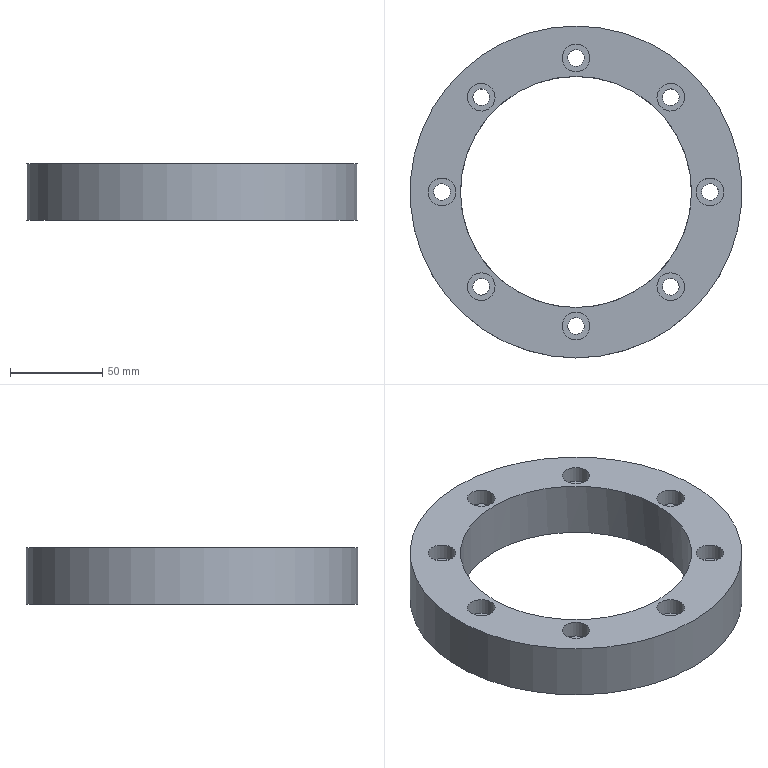Part | NX | features 5003_106_Bearing with gear 2 | 1 solid | 28 faces | box 179.5 x 179.5 x 30.5 mm | volume 373868 mm3 | cylinder 18 | plane 10 | commonest cylinder face diameters 9 x8 15 x8 125 x1 179.5 x1
STEP:
#1=CARTESIAN_POINT('',(66.525,-322.,-216.5));
#2=VERTEX_POINT('',#1);
#3=CARTESIAN_POINT('',(71.025,-322.,-216.5));
#4=DIRECTION('',(0.,0.,1.));
#5=DIRECTION('',(-1.,0.,0.));
#6=AXIS2_PLACEMENT_3D('',#3,#4,#5);
#7=CIRCLE('',#6,4.5);
#8=EDGE_CURVE('',#2,#2,#7,.T.);
#9=ORIENTED_EDGE('',*,*,#8,.T.);
#10=EDGE_LOOP('',(#9));
#11=FACE_BOUND('',#10,.T.);
#12=CARTESIAN_POINT('',(71.025,-317.5,-238.));
#13=VERTEX_POINT('',#12);
#14=CARTESIAN_POINT('',(71.025,-322.,-238.));
#15=DIRECTION('',(0.,0.,-1.));
#16=DIRECTION('',(0.,1.,0.));
#17=AXIS2_PLACEMENT_3D('',#14,#15,#16);
#18=CIRCLE('',#17,4.5);
#19=EDGE_CURVE('',#13,#13,#18,.T.);
#20=ORIENTED_EDGE('',*,*,#19,.T.);
#21=EDGE_LOOP('',(#20));
#22=FACE_BOUND('',#21,.T.);
#23=CARTESIAN_POINT('',(71.025,-322.,-207.5));
#24=DIRECTION('',(0.,0.,1.));
#25=DIRECTION('',(-1.,0.,0.));
#26=AXIS2_PLACEMENT_3D('',#23,#24,#25);
#27=CYLINDRICAL_SURFACE('',#26,4.5);
#28=ADVANCED_FACE('',(#11,#22),#27,.F.);
#29=CARTESIAN_POINT('',(46.608,-370.083,-216.5));
#30=VERTEX_POINT('',#29);
#31=CARTESIAN_POINT('',(49.79,-373.265,-216.5));
#32=DIRECTION('',(0.,0.,1.));
#33=DIRECTION('',(-0.7071,0.7071,0.));
#34=AXIS2_PLACEMENT_3D('',#31,#32,#33);
#35=CIRCLE('',#34,4.5);
#36=EDGE_CURVE('',#30,#30,#35,.T.);
#37=ORIENTED_EDGE('',*,*,#36,.T.);
#38=EDGE_LOOP('',(#37));
#39=FACE_BOUND('',#38,.T.);
#40=CARTESIAN_POINT('',(52.972,-370.083,-238.));
#41=VERTEX_POINT('',#40);
#42=CARTESIAN_POINT('',(49.79,-373.265,-238.));
#43=DIRECTION('',(0.,0.,-1.));
#44=DIRECTION('',(0.7071,0.7071,0.));
#45=AXIS2_PLACEMENT_3D('',#42,#43,#44);
#46=CIRCLE('',#45,4.5);
#47=EDGE_CURVE('',#41,#41,#46,.T.);
#48=ORIENTED_EDGE('',*,*,#47,.T.);
#49=EDGE_LOOP('',(#48));
#50=FACE_BOUND('',#49,.T.);
#51=CARTESIAN_POINT('',(49.79,-373.265,-207.5));
#52=DIRECTION('',(0.,0.,1.));
#53=DIRECTION('',(-0.7071,0.7071,0.));
#54=AXIS2_PLACEMENT_3D('',#51,#52,#53);
#55=CYLINDRICAL_SURFACE('',#54,4.5);
#56=ADVANCED_FACE('',(#39,#50),#55,.F.);
#57=CARTESIAN_POINT('',(-1.475,-390.,-216.5));
#58=VERTEX_POINT('',#57);
#59=CARTESIAN_POINT('',(-1.475,-394.5,-216.5));
#60=DIRECTION('',(0.,0.,1.));
#61=DIRECTION('',(0.,1.,0.));
#62=AXIS2_PLACEMENT_3D('',#59,#60,#61);
#63=CIRCLE('',#62,4.5);
#64=EDGE_CURVE('',#58,#58,#63,.T.);
#65=ORIENTED_EDGE('',*,*,#64,.T.);
#66=EDGE_LOOP('',(#65));
#67=FACE_BOUND('',#66,.T.);
#68=CARTESIAN_POINT('',(3.025,-394.5,-238.));
#69=VERTEX_POINT('',#68);
#70=CARTESIAN_POINT('',(-1.475,-394.5,-238.));
#71=DIRECTION('',(0.,0.,-1.));
#72=DIRECTION('',(1.,0.,0.));
#73=AXIS2_PLACEMENT_3D('',#70,#71,#72);
#74=CIRCLE('',#73,4.5);
#75=EDGE_CURVE('',#69,#69,#74,.T.);
#76=ORIENTED_EDGE('',*,*,#75,.T.);
#77=EDGE_LOOP('',(#76));
#78=FACE_BOUND('',#77,.T.);
#79=CARTESIAN_POINT('',(-1.475,-394.5,-207.5));
#80=DIRECTION('',(0.,0.,1.));
#81=DIRECTION('',(0.,1.,0.));
#82=AXIS2_PLACEMENT_3D('',#79,#80,#81);
#83=CYLINDRICAL_SURFACE('',#82,4.5);
#84=ADVANCED_FACE('',(#67,#78),#83,.F.);
#85=CARTESIAN_POINT('',(-49.558,-370.083,-216.5));
#86=VERTEX_POINT('',#85);
#87=CARTESIAN_POINT('',(-52.74,-373.265,-216.5));
#88=DIRECTION('',(0.,0.,1.));
#89=DIRECTION('',(0.7071,0.7071,0.));
#90=AXIS2_PLACEMENT_3D('',#87,#88,#89);
#91=CIRCLE('',#90,4.5);
#92=EDGE_CURVE('',#86,#86,#91,.T.);
#93=ORIENTED_EDGE('',*,*,#92,.T.);
#94=EDGE_LOOP('',(#93));
#95=FACE_BOUND('',#94,.T.);
#96=CARTESIAN_POINT('',(-49.558,-376.447,-238.));
#97=VERTEX_POINT('',#96);
#98=CARTESIAN_POINT('',(-52.74,-373.265,-238.));
#99=DIRECTION('',(0.,0.,-1.));
#100=DIRECTION('',(0.7071,-0.7071,0.));
#101=AXIS2_PLACEMENT_3D('',#98,#99,#100);
#102=CIRCLE('',#101,4.5);
#103=EDGE_CURVE('',#97,#97,#102,.T.);
#104=ORIENTED_EDGE('',*,*,#103,.T.);
#105=EDGE_LOOP('',(#104));
#106=FACE_BOUND('',#105,.T.);
#107=CARTESIAN_POINT('',(-52.74,-373.265,-207.5));
#108=DIRECTION('',(0.,0.,1.));
#109=DIRECTION('',(0.7071,0.7071,0.));
#110=AXIS2_PLACEMENT_3D('',#107,#108,#109);
#111=CYLINDRICAL_SURFACE('',#110,4.5);
#112=ADVANCED_FACE('',(#95,#106),#111,.F.);
#113=CARTESIAN_POINT('',(-69.475,-322.,-216.5));
#114=VERTEX_POINT('',#113);
#115=CARTESIAN_POINT('',(-73.975,-322.,-216.5));
#116=DIRECTION('',(0.,0.,1.));
#117=DIRECTION('',(1.,0.,0.));
#118=AXIS2_PLACEMENT_3D('',#115,#116,#117);
#119=CIRCLE('',#118,4.5);
#120=EDGE_CURVE('',#114,#114,#119,.T.);
#121=ORIENTED_EDGE('',*,*,#120,.T.);
#122=EDGE_LOOP('',(#121));
#123=FACE_BOUND('',#122,.T.);
#124=CARTESIAN_POINT('',(-73.975,-326.5,-238.));
#125=VERTEX_POINT('',#124);
#126=CARTESIAN_POINT('',(-73.975,-322.,-238.));
#127=DIRECTION('',(0.,0.,-1.));
#128=DIRECTION('',(0.,-1.,0.));
#129=AXIS2_PLACEMENT_3D('',#126,#127,#128);
#130=CIRCLE('',#129,4.5);
#131=EDGE_CURVE('',#125,#125,#130,.T.);
#132=ORIENTED_EDGE('',*,*,#131,.T.);
#133=EDGE_LOOP('',(#132));
#134=FACE_BOUND('',#133,.T.);
#135=CARTESIAN_POINT('',(-73.975,-322.,-207.5));
#136=DIRECTION('',(0.,0.,1.));
#137=DIRECTION('',(1.,0.,0.));
#138=AXIS2_PLACEMENT_3D('',#135,#136,#137);
#139=CYLINDRICAL_SURFACE('',#138,4.5);
#140=ADVANCED_FACE('',(#123,#134),#139,.F.);
#141=CARTESIAN_POINT('',(-49.558,-273.917,-216.5));
#142=VERTEX_POINT('',#141);
#143=CARTESIAN_POINT('',(-52.74,-270.735,-216.5));
#144=DIRECTION('',(0.,0.,1.));
#145=DIRECTION('',(0.7071,-0.7071,0.));
#146=AXIS2_PLACEMENT_3D('',#143,#144,#145);
#147=CIRCLE('',#146,4.5);
#148=EDGE_CURVE('',#142,#142,#147,.T.);
#149=ORIENTED_EDGE('',*,*,#148,.T.);
#150=EDGE_LOOP('',(#149));
#151=FACE_BOUND('',#150,.T.);
#152=CARTESIAN_POINT('',(-55.922,-273.917,-238.));
#153=VERTEX_POINT('',#152);
#154=CARTESIAN_POINT('',(-52.74,-270.735,-238.));
#155=DIRECTION('',(0.,0.,-1.));
#156=DIRECTION('',(-0.7071,-0.7071,0.));
#157=AXIS2_PLACEMENT_3D('',#154,#155,#156);
#158=CIRCLE('',#157,4.5);
#159=EDGE_CURVE('',#153,#153,#158,.T.);
#160=ORIENTED_EDGE('',*,*,#159,.T.);
#161=EDGE_LOOP('',(#160));
#162=FACE_BOUND('',#161,.T.);
#163=CARTESIAN_POINT('',(-52.74,-270.735,-207.5));
#164=DIRECTION('',(0.,0.,1.));
#165=DIRECTION('',(0.7071,-0.7071,0.));
#166=AXIS2_PLACEMENT_3D('',#163,#164,#165);
#167=CYLINDRICAL_SURFACE('',#166,4.5);
#168=ADVANCED_FACE('',(#151,#162),#167,.F.);
#169=CARTESIAN_POINT('',(-1.475,-254.,-216.5));
#170=VERTEX_POINT('',#169);
#171=CARTESIAN_POINT('',(-1.475,-249.5,-216.5));
#172=DIRECTION('',(0.,0.,1.));
#173=DIRECTION('',(0.,-1.,0.));
#174=AXIS2_PLACEMENT_3D('',#171,#172,#173);
#175=CIRCLE('',#174,4.5);
#176=EDGE_CURVE('',#170,#170,#175,.T.);
#177=ORIENTED_EDGE('',*,*,#176,.T.);
#178=EDGE_LOOP('',(#177));
#179=FACE_BOUND('',#178,.T.);
#180=CARTESIAN_POINT('',(-5.975,-249.5,-238.));
#181=VERTEX_POINT('',#180);
#182=CARTESIAN_POINT('',(-1.475,-249.5,-238.));
#183=DIRECTION('',(0.,0.,-1.));
#184=DIRECTION('',(-1.,0.,0.));
#185=AXIS2_PLACEMENT_3D('',#182,#183,#184);
#186=CIRCLE('',#185,4.5);
#187=EDGE_CURVE('',#181,#181,#186,.T.);
#188=ORIENTED_EDGE('',*,*,#187,.T.);
#189=EDGE_LOOP('',(#188));
#190=FACE_BOUND('',#189,.T.);
#191=CARTESIAN_POINT('',(-1.475,-249.5,-207.5));
#192=DIRECTION('',(0.,0.,1.));
#193=DIRECTION('',(0.,-1.,0.));
#194=AXIS2_PLACEMENT_3D('',#191,#192,#193);
#195=CYLINDRICAL_SURFACE('',#194,4.5);
#196=ADVANCED_FACE('',(#179,#190),#195,.F.);
#197=CARTESIAN_POINT('',(46.608,-273.917,-216.5));
#198=VERTEX_POINT('',#197);
#199=CARTESIAN_POINT('',(49.79,-270.735,-216.5));
#200=DIRECTION('',(0.,0.,1.));
#201=DIRECTION('',(-0.7071,-0.7071,0.));
#202=AXIS2_PLACEMENT_3D('',#199,#200,#201);
#203=CIRCLE('',#202,4.5);
#204=EDGE_CURVE('',#198,#198,#203,.T.);
#205=ORIENTED_EDGE('',*,*,#204,.T.);
#206=EDGE_LOOP('',(#205));
#207=FACE_BOUND('',#206,.T.);
#208=CARTESIAN_POINT('',(46.608,-267.553,-238.));
#209=VERTEX_POINT('',#208);
#210=CARTESIAN_POINT('',(49.79,-270.735,-238.));
#211=DIRECTION('',(0.,0.,-1.));
#212=DIRECTION('',(-0.7071,0.7071,0.));
#213=AXIS2_PLACEMENT_3D('',#210,#211,#212);
#214=CIRCLE('',#213,4.5);
#215=EDGE_CURVE('',#209,#209,#214,.T.);
#216=ORIENTED_EDGE('',*,*,#215,.T.);
#217=EDGE_LOOP('',(#216));
#218=FACE_BOUND('',#217,.T.);
#219=CARTESIAN_POINT('',(49.79,-270.735,-207.5));
#220=DIRECTION('',(0.,0.,1.));
#221=DIRECTION('',(-0.7071,-0.7071,0.));
#222=AXIS2_PLACEMENT_3D('',#219,#220,#221);
#223=CYLINDRICAL_SURFACE('',#222,4.5);
#224=ADVANCED_FACE('',(#207,#218),#223,.F.);
#225=ORIENTED_EDGE('',*,*,#8,.F.);
#226=EDGE_LOOP('',(#225));
#227=FACE_BOUND('',#226,.T.);
#228=CARTESIAN_POINT('',(63.525,-322.,-216.5));
#229=VERTEX_POINT('',#228);
#230=CARTESIAN_POINT('',(71.025,-322.,-216.5));
#231=DIRECTION('',(0.,0.,1.));
#232=DIRECTION('',(-1.,0.,0.));
#233=AXIS2_PLACEMENT_3D('',#230,#231,#232);
#234=CIRCLE('',#233,7.5);
#235=EDGE_CURVE('',#229,#229,#234,.T.);
#236=ORIENTED_EDGE('',*,*,#235,.T.);
#237=EDGE_LOOP('',(#236));
#238=FACE_BOUND('',#237,.T.);
#239=CARTESIAN_POINT('',(71.025,-326.5,-216.5));
#240=DIRECTION('',(0.,0.,-1.));
#241=DIRECTION('',(1.,0.,0.));
#242=AXIS2_PLACEMENT_3D('',#239,#240,#241);
#243=PLANE('',#242);
#244=ADVANCED_FACE('',(#227,#238),#243,.F.);
#245=ORIENTED_EDGE('',*,*,#36,.F.);
#246=EDGE_LOOP('',(#245));
#247=FACE_BOUND('',#246,.T.);
#248=CARTESIAN_POINT('',(44.487,-367.962,-216.5));
#249=VERTEX_POINT('',#248);
#250=CARTESIAN_POINT('',(49.79,-373.265,-216.5));
#251=DIRECTION('',(0.,0.,1.));
#252=DIRECTION('',(-0.7071,0.7071,0.));
#253=AXIS2_PLACEMENT_3D('',#250,#251,#252);
#254=CIRCLE('',#253,7.5);
#255=EDGE_CURVE('',#249,#249,#254,.T.);
#256=ORIENTED_EDGE('',*,*,#255,.T.);
#257=EDGE_LOOP('',(#256));
#258=FACE_BOUND('',#257,.T.);
#259=CARTESIAN_POINT('',(46.608,-376.447,-216.5));
#260=DIRECTION('',(0.,0.,-1.));
#261=DIRECTION('',(0.7071,-0.7071,0.));
#262=AXIS2_PLACEMENT_3D('',#259,#260,#261);
#263=PLANE('',#262);
#264=ADVANCED_FACE('',(#247,#258),#263,.F.);
#265=ORIENTED_EDGE('',*,*,#64,.F.);
#266=EDGE_LOOP('',(#265));
#267=FACE_BOUND('',#266,.T.);
#268=CARTESIAN_POINT('',(-1.475,-387.,-216.5));
#269=VERTEX_POINT('',#268);
#270=CARTESIAN_POINT('',(-1.475,-394.5,-216.5));
#271=DIRECTION('',(0.,0.,1.));
#272=DIRECTION('',(0.,1.,0.));
#273=AXIS2_PLACEMENT_3D('',#270,#271,#272);
#274=CIRCLE('',#273,7.5);
#275=EDGE_CURVE('',#269,#269,#274,.T.);
#276=ORIENTED_EDGE('',*,*,#275,.T.);
#277=EDGE_LOOP('',(#276));
#278=FACE_BOUND('',#277,.T.);
#279=CARTESIAN_POINT('',(-5.975,-394.5,-216.5));
#280=DIRECTION('',(0.,0.,-1.));
#281=DIRECTION('',(0.,-1.,0.));
#282=AXIS2_PLACEMENT_3D('',#279,#280,#281);
#283=PLANE('',#282);
#284=ADVANCED_FACE('',(#267,#278),#283,.F.);
#285=ORIENTED_EDGE('',*,*,#92,.F.);
#286=EDGE_LOOP('',(#285));
#287=FACE_BOUND('',#286,.T.);
#288=CARTESIAN_POINT('',(-47.437,-367.962,-216.5));
#289=VERTEX_POINT('',#288);
#290=CARTESIAN_POINT('',(-52.74,-373.265,-216.5));
#291=DIRECTION('',(0.,0.,1.));
#292=DIRECTION('',(0.7071,0.7071,0.));
#293=AXIS2_PLACEMENT_3D('',#290,#291,#292);
#294=CIRCLE('',#293,7.5);
#295=EDGE_CURVE('',#289,#289,#294,.T.);
#296=ORIENTED_EDGE('',*,*,#295,.T.);
#297=EDGE_LOOP('',(#296));
#298=FACE_BOUND('',#297,.T.);
#299=CARTESIAN_POINT('',(-55.922,-370.083,-216.5));
#300=DIRECTION('',(0.,0.,-1.));
#301=DIRECTION('',(-0.7071,-0.7071,0.));
#302=AXIS2_PLACEMENT_3D('',#299,#300,#301);
#303=PLANE('',#302);
#304=ADVANCED_FACE('',(#287,#298),#303,.F.);
#305=ORIENTED_EDGE('',*,*,#120,.F.);
#306=EDGE_LOOP('',(#305));
#307=FACE_BOUND('',#306,.T.);
#308=CARTESIAN_POINT('',(-66.475,-322.,-216.5));
#309=VERTEX_POINT('',#308);
#310=CARTESIAN_POINT('',(-73.975,-322.,-216.5));
#311=DIRECTION('',(0.,0.,1.));
#312=DIRECTION('',(1.,0.,0.));
#313=AXIS2_PLACEMENT_3D('',#310,#311,#312);
#314=CIRCLE('',#313,7.5);
#315=EDGE_CURVE('',#309,#309,#314,.T.);
#316=ORIENTED_EDGE('',*,*,#315,.T.);
#317=EDGE_LOOP('',(#316));
#318=FACE_BOUND('',#317,.T.);
#319=CARTESIAN_POINT('',(-73.975,-317.5,-216.5));
#320=DIRECTION('',(0.,0.,-1.));
#321=DIRECTION('',(-1.,0.,0.));
#322=AXIS2_PLACEMENT_3D('',#319,#320,#321);
#323=PLANE('',#322);
#324=ADVANCED_FACE('',(#307,#318),#323,.F.);
#325=ORIENTED_EDGE('',*,*,#148,.F.);
#326=EDGE_LOOP('',(#325));
#327=FACE_BOUND('',#326,.T.);
#328=CARTESIAN_POINT('',(-47.437,-276.038,-216.5));
#329=VERTEX_POINT('',#328);
#330=CARTESIAN_POINT('',(-52.74,-270.735,-216.5));
#331=DIRECTION('',(0.,0.,1.));
#332=DIRECTION('',(0.7071,-0.7071,0.));
#333=AXIS2_PLACEMENT_3D('',#330,#331,#332);
#334=CIRCLE('',#333,7.5);
#335=EDGE_CURVE('',#329,#329,#334,.T.);
#336=ORIENTED_EDGE('',*,*,#335,.T.);
#337=EDGE_LOOP('',(#336));
#338=FACE_BOUND('',#337,.T.);
#339=CARTESIAN_POINT('',(-49.558,-267.553,-216.5));
#340=DIRECTION('',(0.,0.,-1.));
#341=DIRECTION('',(-0.7071,0.7071,0.));
#342=AXIS2_PLACEMENT_3D('',#339,#340,#341);
#343=PLANE('',#342);
#344=ADVANCED_FACE('',(#327,#338),#343,.F.);
#345=ORIENTED_EDGE('',*,*,#176,.F.);
#346=EDGE_LOOP('',(#345));
#347=FACE_BOUND('',#346,.T.);
#348=CARTESIAN_POINT('',(-1.475,-257.,-216.5));
#349=VERTEX_POINT('',#348);
#350=CARTESIAN_POINT('',(-1.475,-249.5,-216.5));
#351=DIRECTION('',(0.,0.,1.));
#352=DIRECTION('',(0.,-1.,0.));
#353=AXIS2_PLACEMENT_3D('',#350,#351,#352);
#354=CIRCLE('',#353,7.5);
#355=EDGE_CURVE('',#349,#349,#354,.T.);
#356=ORIENTED_EDGE('',*,*,#355,.T.);
#357=EDGE_LOOP('',(#356));
#358=FACE_BOUND('',#357,.T.);
#359=CARTESIAN_POINT('',(3.025,-249.5,-216.5));
#360=DIRECTION('',(0.,0.,-1.));
#361=DIRECTION('',(0.,1.,0.));
#362=AXIS2_PLACEMENT_3D('',#359,#360,#361);
#363=PLANE('',#362);
#364=ADVANCED_FACE('',(#347,#358),#363,.F.);
#365=ORIENTED_EDGE('',*,*,#204,.F.);
#366=EDGE_LOOP('',(#365));
#367=FACE_BOUND('',#366,.T.);
#368=CARTESIAN_POINT('',(44.487,-276.038,-216.5));
#369=VERTEX_POINT('',#368);
#370=CARTESIAN_POINT('',(49.79,-270.735,-216.5));
#371=DIRECTION('',(0.,0.,1.));
#372=DIRECTION('',(-0.7071,-0.7071,0.));
#373=AXIS2_PLACEMENT_3D('',#370,#371,#372);
#374=CIRCLE('',#373,7.5);
#375=EDGE_CURVE('',#369,#369,#374,.T.);
#376=ORIENTED_EDGE('',*,*,#375,.T.);
#377=EDGE_LOOP('',(#376));
#378=FACE_BOUND('',#377,.T.);
#379=CARTESIAN_POINT('',(52.972,-273.917,-216.5));
#380=DIRECTION('',(0.,0.,-1.));
#381=DIRECTION('',(0.7071,0.7071,0.));
#382=AXIS2_PLACEMENT_3D('',#379,#380,#381);
#383=PLANE('',#382);
#384=ADVANCED_FACE('',(#367,#378),#383,.F.);
#385=CARTESIAN_POINT('',(-1.475,-259.5,-238.));
#386=VERTEX_POINT('',#385);
#387=CARTESIAN_POINT('',(-1.475,-322.,-238.));
#388=DIRECTION('',(0.,0.,-1.));
#389=DIRECTION('',(0.,1.,0.));
#390=AXIS2_PLACEMENT_3D('',#387,#388,#389);
#391=CIRCLE('',#390,62.5);
#392=EDGE_CURVE('',#386,#386,#391,.T.);
#393=ORIENTED_EDGE('',*,*,#392,.T.);
#394=EDGE_LOOP('',(#393));
#395=FACE_BOUND('',#394,.T.);
#396=CARTESIAN_POINT('',(-1.475,-384.5,-207.5));
#397=VERTEX_POINT('',#396);
#398=CARTESIAN_POINT('',(-1.475,-322.,-207.5));
#399=DIRECTION('',(0.,0.,1.));
#400=DIRECTION('',(0.,-1.,0.));
#401=AXIS2_PLACEMENT_3D('',#398,#399,#400);
#402=CIRCLE('',#401,62.5);
#403=EDGE_CURVE('',#397,#397,#402,.F.);
#404=ORIENTED_EDGE('',*,*,#403,.F.);
#405=EDGE_LOOP('',(#404));
#406=FACE_BOUND('',#405,.T.);
#407=CARTESIAN_POINT('',(-1.475,-322.,-202.));
#408=DIRECTION('',(0.,0.,-1.));
#409=DIRECTION('',(0.,1.,0.));
#410=AXIS2_PLACEMENT_3D('',#407,#408,#409);
#411=CYLINDRICAL_SURFACE('',#410,62.5);
#412=ADVANCED_FACE('',(#395,#406),#411,.F.);
#413=ORIENTED_EDGE('',*,*,#235,.F.);
#414=EDGE_LOOP('',(#413));
#415=FACE_BOUND('',#414,.T.);
#416=CARTESIAN_POINT('',(63.525,-322.,-207.5));
#417=VERTEX_POINT('',#416);
#418=CARTESIAN_POINT('',(71.025,-322.,-207.5));
#419=DIRECTION('',(0.,0.,1.));
#420=DIRECTION('',(-1.,0.,0.));
#421=AXIS2_PLACEMENT_3D('',#418,#419,#420);
#422=CIRCLE('',#421,7.5);
#423=EDGE_CURVE('',#417,#417,#422,.T.);
#424=ORIENTED_EDGE('',*,*,#423,.T.);
#425=EDGE_LOOP('',(#424));
#426=FACE_BOUND('',#425,.T.);
#427=CARTESIAN_POINT('',(71.025,-322.,-207.5));
#428=DIRECTION('',(0.,0.,1.));
#429=DIRECTION('',(-1.,0.,0.));
#430=AXIS2_PLACEMENT_3D('',#427,#428,#429);
#431=CYLINDRICAL_SURFACE('',#430,7.5);
#432=ADVANCED_FACE('',(#415,#426),#431,.F.);
#433=ORIENTED_EDGE('',*,*,#255,.F.);
#434=EDGE_LOOP('',(#433));
#435=FACE_BOUND('',#434,.T.);
#436=CARTESIAN_POINT('',(44.487,-367.962,-207.5));
#437=VERTEX_POINT('',#436);
#438=CARTESIAN_POINT('',(49.79,-373.265,-207.5));
#439=DIRECTION('',(0.,0.,1.));
#440=DIRECTION('',(-0.7071,0.7071,0.));
#441=AXIS2_PLACEMENT_3D('',#438,#439,#440);
#442=CIRCLE('',#441,7.5);
#443=EDGE_CURVE('',#437,#437,#442,.T.);
#444=ORIENTED_EDGE('',*,*,#443,.T.);
#445=EDGE_LOOP('',(#444));
#446=FACE_BOUND('',#445,.T.);
#447=CARTESIAN_POINT('',(49.79,-373.265,-207.5));
#448=DIRECTION('',(0.,0.,1.));
#449=DIRECTION('',(-0.7071,0.7071,0.));
#450=AXIS2_PLACEMENT_3D('',#447,#448,#449);
#451=CYLINDRICAL_SURFACE('',#450,7.5);
#452=ADVANCED_FACE('',(#435,#446),#451,.F.);
#453=ORIENTED_EDGE('',*,*,#275,.F.);
#454=EDGE_LOOP('',(#453));
#455=FACE_BOUND('',#454,.T.);
#456=CARTESIAN_POINT('',(-1.475,-387.,-207.5));
#457=VERTEX_POINT('',#456);
#458=CARTESIAN_POINT('',(-1.475,-394.5,-207.5));
#459=DIRECTION('',(0.,0.,1.));
#460=DIRECTION('',(0.,1.,0.));
#461=AXIS2_PLACEMENT_3D('',#458,#459,#460);
#462=CIRCLE('',#461,7.5);
#463=EDGE_CURVE('',#457,#457,#462,.T.);
#464=ORIENTED_EDGE('',*,*,#463,.T.);
#465=EDGE_LOOP('',(#464));
#466=FACE_BOUND('',#465,.T.);
#467=CARTESIAN_POINT('',(-1.475,-394.5,-207.5));
#468=DIRECTION('',(0.,0.,1.));
#469=DIRECTION('',(0.,1.,0.));
#470=AXIS2_PLACEMENT_3D('',#467,#468,#469);
#471=CYLINDRICAL_SURFACE('',#470,7.5);
#472=ADVANCED_FACE('',(#455,#466),#471,.F.);
#473=ORIENTED_EDGE('',*,*,#295,.F.);
#474=EDGE_LOOP('',(#473));
#475=FACE_BOUND('',#474,.T.);
#476=CARTESIAN_POINT('',(-47.437,-367.962,-207.5));
#477=VERTEX_POINT('',#476);
#478=CARTESIAN_POINT('',(-52.74,-373.265,-207.5));
#479=DIRECTION('',(0.,0.,1.));
#480=DIRECTION('',(0.7071,0.7071,0.));
#481=AXIS2_PLACEMENT_3D('',#478,#479,#480);
#482=CIRCLE('',#481,7.5);
#483=EDGE_CURVE('',#477,#477,#482,.T.);
#484=ORIENTED_EDGE('',*,*,#483,.T.);
#485=EDGE_LOOP('',(#484));
#486=FACE_BOUND('',#485,.T.);
#487=CARTESIAN_POINT('',(-52.74,-373.265,-207.5));
#488=DIRECTION('',(0.,0.,1.));
#489=DIRECTION('',(0.7071,0.7071,0.));
#490=AXIS2_PLACEMENT_3D('',#487,#488,#489);
#491=CYLINDRICAL_SURFACE('',#490,7.5);
#492=ADVANCED_FACE('',(#475,#486),#491,.F.);
#493=ORIENTED_EDGE('',*,*,#315,.F.);
#494=EDGE_LOOP('',(#493));
#495=FACE_BOUND('',#494,.T.);
#496=CARTESIAN_POINT('',(-66.475,-322.,-207.5));
#497=VERTEX_POINT('',#496);
#498=CARTESIAN_POINT('',(-73.975,-322.,-207.5));
#499=DIRECTION('',(0.,0.,1.));
#500=DIRECTION('',(1.,0.,0.));
#501=AXIS2_PLACEMENT_3D('',#498,#499,#500);
#502=CIRCLE('',#501,7.5);
#503=EDGE_CURVE('',#497,#497,#502,.T.);
#504=ORIENTED_EDGE('',*,*,#503,.T.);
#505=EDGE_LOOP('',(#504));
#506=FACE_BOUND('',#505,.T.);
#507=CARTESIAN_POINT('',(-73.975,-322.,-207.5));
#508=DIRECTION('',(0.,0.,1.));
#509=DIRECTION('',(1.,0.,0.));
#510=AXIS2_PLACEMENT_3D('',#507,#508,#509);
#511=CYLINDRICAL_SURFACE('',#510,7.5);
#512=ADVANCED_FACE('',(#495,#506),#511,.F.);
#513=ORIENTED_EDGE('',*,*,#335,.F.);
#514=EDGE_LOOP('',(#513));
#515=FACE_BOUND('',#514,.T.);
#516=CARTESIAN_POINT('',(-47.437,-276.038,-207.5));
#517=VERTEX_POINT('',#516);
#518=CARTESIAN_POINT('',(-52.74,-270.735,-207.5));
#519=DIRECTION('',(0.,0.,1.));
#520=DIRECTION('',(0.7071,-0.7071,0.));
#521=AXIS2_PLACEMENT_3D('',#518,#519,#520);
#522=CIRCLE('',#521,7.5);
#523=EDGE_CURVE('',#517,#517,#522,.T.);
#524=ORIENTED_EDGE('',*,*,#523,.T.);
#525=EDGE_LOOP('',(#524));
#526=FACE_BOUND('',#525,.T.);
#527=CARTESIAN_POINT('',(-52.74,-270.735,-207.5));
#528=DIRECTION('',(0.,0.,1.));
#529=DIRECTION('',(0.7071,-0.7071,0.));
#530=AXIS2_PLACEMENT_3D('',#527,#528,#529);
#531=CYLINDRICAL_SURFACE('',#530,7.5);
#532=ADVANCED_FACE('',(#515,#526),#531,.F.);
#533=ORIENTED_EDGE('',*,*,#355,.F.);
#534=EDGE_LOOP('',(#533));
#535=FACE_BOUND('',#534,.T.);
#536=CARTESIAN_POINT('',(-1.475,-257.,-207.5));
#537=VERTEX_POINT('',#536);
#538=CARTESIAN_POINT('',(-1.475,-249.5,-207.5));
#539=DIRECTION('',(0.,0.,1.));
#540=DIRECTION('',(0.,-1.,0.));
#541=AXIS2_PLACEMENT_3D('',#538,#539,#540);
#542=CIRCLE('',#541,7.5);
#543=EDGE_CURVE('',#537,#537,#542,.T.);
#544=ORIENTED_EDGE('',*,*,#543,.T.);
#545=EDGE_LOOP('',(#544));
#546=FACE_BOUND('',#545,.T.);
#547=CARTESIAN_POINT('',(-1.475,-249.5,-207.5));
#548=DIRECTION('',(0.,0.,1.));
#549=DIRECTION('',(0.,-1.,0.));
#550=AXIS2_PLACEMENT_3D('',#547,#548,#549);
#551=CYLINDRICAL_SURFACE('',#550,7.5);
#552=ADVANCED_FACE('',(#535,#546),#551,.F.);
#553=ORIENTED_EDGE('',*,*,#375,.F.);
#554=EDGE_LOOP('',(#553));
#555=FACE_BOUND('',#554,.T.);
#556=CARTESIAN_POINT('',(44.487,-276.038,-207.5));
#557=VERTEX_POINT('',#556);
#558=CARTESIAN_POINT('',(49.79,-270.735,-207.5));
#559=DIRECTION('',(0.,0.,1.));
#560=DIRECTION('',(-0.7071,-0.7071,0.));
#561=AXIS2_PLACEMENT_3D('',#558,#559,#560);
#562=CIRCLE('',#561,7.5);
#563=EDGE_CURVE('',#557,#557,#562,.T.);
#564=ORIENTED_EDGE('',*,*,#563,.T.);
#565=EDGE_LOOP('',(#564));
#566=FACE_BOUND('',#565,.T.);
#567=CARTESIAN_POINT('',(49.79,-270.735,-207.5));
#568=DIRECTION('',(0.,0.,1.));
#569=DIRECTION('',(-0.7071,-0.7071,0.));
#570=AXIS2_PLACEMENT_3D('',#567,#568,#569);
#571=CYLINDRICAL_SURFACE('',#570,7.5);
#572=ADVANCED_FACE('',(#555,#566),#571,.F.);
#573=ORIENTED_EDGE('',*,*,#563,.F.);
#574=EDGE_LOOP('',(#573));
#575=FACE_BOUND('',#574,.T.);
#576=ORIENTED_EDGE('',*,*,#543,.F.);
#577=EDGE_LOOP('',(#576));
#578=FACE_BOUND('',#577,.T.);
#579=ORIENTED_EDGE('',*,*,#523,.F.);
#580=EDGE_LOOP('',(#579));
#581=FACE_BOUND('',#580,.T.);
#582=ORIENTED_EDGE('',*,*,#503,.F.);
#583=EDGE_LOOP('',(#582));
#584=FACE_BOUND('',#583,.T.);
#585=ORIENTED_EDGE('',*,*,#483,.F.);
#586=EDGE_LOOP('',(#585));
#587=FACE_BOUND('',#586,.T.);
#588=ORIENTED_EDGE('',*,*,#463,.F.);
#589=EDGE_LOOP('',(#588));
#590=FACE_BOUND('',#589,.T.);
#591=ORIENTED_EDGE('',*,*,#443,.F.);
#592=EDGE_LOOP('',(#591));
#593=FACE_BOUND('',#592,.T.);
#594=ORIENTED_EDGE('',*,*,#423,.F.);
#595=EDGE_LOOP('',(#594));
#596=FACE_BOUND('',#595,.T.);
#597=CARTESIAN_POINT('',(-1.475,-411.75,-207.5));
#598=VERTEX_POINT('',#597);
#599=CARTESIAN_POINT('',(-1.475,-322.,-207.5));
#600=DIRECTION('',(0.,0.,1.));
#601=DIRECTION('',(0.,-1.,0.));
#602=AXIS2_PLACEMENT_3D('',#599,#600,#601);
#603=CIRCLE('',#602,89.75);
#604=EDGE_CURVE('',#598,#598,#603,.T.);
#605=ORIENTED_EDGE('',*,*,#604,.T.);
#606=EDGE_LOOP('',(#605));
#607=FACE_BOUND('',#606,.T.);
#608=ORIENTED_EDGE('',*,*,#403,.T.);
#609=EDGE_LOOP('',(#608));
#610=FACE_BOUND('',#609,.T.);
#611=CARTESIAN_POINT('',(-1.475,-322.,-207.5));
#612=DIRECTION('',(0.,0.,1.));
#613=DIRECTION('',(0.,-1.,0.));
#614=AXIS2_PLACEMENT_3D('',#611,#612,#613);
#615=PLANE('',#614);
#616=ADVANCED_FACE('',(#575,#578,#581,#584,#587,#590,#593,#596,#607,#610),#615,.T.);
#617=ORIENTED_EDGE('',*,*,#215,.F.);
#618=EDGE_LOOP('',(#617));
#619=FACE_BOUND('',#618,.T.);
#620=ORIENTED_EDGE('',*,*,#187,.F.);
#621=EDGE_LOOP('',(#620));
#622=FACE_BOUND('',#621,.T.);
#623=ORIENTED_EDGE('',*,*,#159,.F.);
#624=EDGE_LOOP('',(#623));
#625=FACE_BOUND('',#624,.T.);
#626=ORIENTED_EDGE('',*,*,#131,.F.);
#627=EDGE_LOOP('',(#626));
#628=FACE_BOUND('',#627,.T.);
#629=ORIENTED_EDGE('',*,*,#103,.F.);
#630=EDGE_LOOP('',(#629));
#631=FACE_BOUND('',#630,.T.);
#632=ORIENTED_EDGE('',*,*,#75,.F.);
#633=EDGE_LOOP('',(#632));
#634=FACE_BOUND('',#633,.T.);
#635=ORIENTED_EDGE('',*,*,#47,.F.);
#636=EDGE_LOOP('',(#635));
#637=FACE_BOUND('',#636,.T.);
#638=ORIENTED_EDGE('',*,*,#19,.F.);
#639=EDGE_LOOP('',(#638));
#640=FACE_BOUND('',#639,.T.);
#641=ORIENTED_EDGE('',*,*,#392,.F.);
#642=EDGE_LOOP('',(#641));
#643=FACE_BOUND('',#642,.T.);
#644=CARTESIAN_POINT('',(-1.475,-232.25,-238.));
#645=VERTEX_POINT('',#644);
#646=CARTESIAN_POINT('',(-1.475,-322.,-238.));
#647=DIRECTION('',(0.,0.,-1.));
#648=DIRECTION('',(0.,1.,0.));
#649=AXIS2_PLACEMENT_3D('',#646,#647,#648);
#650=CIRCLE('',#649,89.75);
#651=EDGE_CURVE('',#645,#645,#650,.T.);
#652=ORIENTED_EDGE('',*,*,#651,.T.);
#653=EDGE_LOOP('',(#652));
#654=FACE_BOUND('',#653,.T.);
#655=CARTESIAN_POINT('',(-1.475,-322.,-238.));
#656=DIRECTION('',(0.,0.,-1.));
#657=DIRECTION('',(0.,1.,0.));
#658=AXIS2_PLACEMENT_3D('',#655,#656,#657);
#659=PLANE('',#658);
#660=ADVANCED_FACE('',(#619,#622,#625,#628,#631,#634,#637,#640,#643,#654),#659,.T.);
#661=ORIENTED_EDGE('',*,*,#651,.F.);
#662=EDGE_LOOP('',(#661));
#663=FACE_BOUND('',#662,.T.);
#664=ORIENTED_EDGE('',*,*,#604,.F.);
#665=EDGE_LOOP('',(#664));
#666=FACE_BOUND('',#665,.T.);
#667=CARTESIAN_POINT('',(-1.475,-322.,-232.5));
#668=DIRECTION('',(0.,0.,-1.));
#669=DIRECTION('',(0.,1.,0.));
#670=AXIS2_PLACEMENT_3D('',#667,#668,#669);
#671=CYLINDRICAL_SURFACE('',#670,89.75);
#672=ADVANCED_FACE('',(#663,#666),#671,.T.);
#673=CLOSED_SHELL('',(#28,#56,#84,#112,#140,#168,#196,#224,#244,#264,#284,#304,#324,#344,#364,#384,#412,#432,#452,#472,#492,#512,#532,#552,#572,#616,#660,#672));
#674=MANIFOLD_SOLID_BREP('',#673);
#675=(LENGTH_UNIT()NAMED_UNIT(*)SI_UNIT(.MILLI.,.METRE.));
#676=UNCERTAINTY_MEASURE_WITH_UNIT(LENGTH_MEASURE(0.00001),#675,'','');
#677=(NAMED_UNIT(*)PLANE_ANGLE_UNIT()SI_UNIT($,.RADIAN.));
#678=(NAMED_UNIT(*)SI_UNIT($,.STERADIAN.)SOLID_ANGLE_UNIT());
#679=(GEOMETRIC_REPRESENTATION_CONTEXT(3)GLOBAL_UNCERTAINTY_ASSIGNED_CONTEXT((#676))GLOBAL_UNIT_ASSIGNED_CONTEXT((#675,#677,#678))REPRESENTATION_CONTEXT('',''));
#680=ADVANCED_BREP_SHAPE_REPRESENTATION('',(#674),#679);